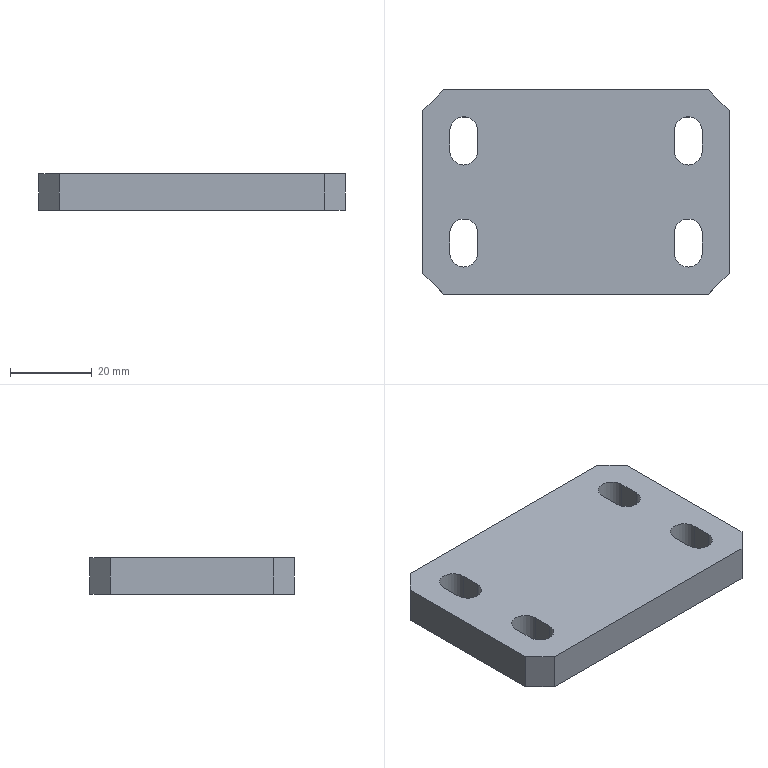Part | STEP file | [03]-6 | 1 solid | 30 faces | box 75 x 50 x 9 mm | volume 30769 mm3 | plane 18 | cylinder 12 | commonest cylinder face diameters 6.8 x12
STEP:
#1=CARTESIAN_POINT('',(65.,6.6,9.));
#2=VERTEX_POINT('',#1);
#3=CARTESIAN_POINT('',(61.6,10.,9.));
#4=VERTEX_POINT('',#3);
#5=CARTESIAN_POINT('',(65.,10.,9.));
#6=DIRECTION('',(0.,0.,-1.));
#7=DIRECTION('',(0.,-1.,0.));
#8=AXIS2_PLACEMENT_3D('',#5,#6,#7);
#9=CIRCLE('',#8,3.4);
#10=EDGE_CURVE('',#2,#4,#9,.T.);
#11=ORIENTED_EDGE('',*,*,#10,.F.);
#12=CARTESIAN_POINT('',(65.,6.6,0.));
#13=VERTEX_POINT('',#12);
#14=CARTESIAN_POINT('',(65.,6.6,9.));
#15=DIRECTION('',(0.,0.,-1.));
#16=VECTOR('',#15,1000.);
#17=LINE('',#14,#16);
#18=EDGE_CURVE('',#2,#13,#17,.T.);
#19=ORIENTED_EDGE('',*,*,#18,.T.);
#20=CARTESIAN_POINT('',(61.6,10.,0.));
#21=VERTEX_POINT('',#20);
#22=CARTESIAN_POINT('',(65.,10.,0.));
#23=DIRECTION('',(0.,0.,1.));
#24=DIRECTION('',(0.,1.,0.));
#25=AXIS2_PLACEMENT_3D('',#22,#23,#24);
#26=CIRCLE('',#25,3.4);
#27=EDGE_CURVE('',#21,#13,#26,.T.);
#28=ORIENTED_EDGE('',*,*,#27,.F.);
#29=CARTESIAN_POINT('',(61.6,10.,9.));
#30=DIRECTION('',(0.,0.,-1.));
#31=VECTOR('',#30,1000.);
#32=LINE('',#29,#31);
#33=EDGE_CURVE('',#4,#21,#32,.T.);
#34=ORIENTED_EDGE('',*,*,#33,.F.);
#35=EDGE_LOOP('',(#11,#19,#28,#34));
#36=FACE_OUTER_BOUND('',#35,.T.);
#37=CARTESIAN_POINT('',(65.,10.,9.));
#38=DIRECTION('',(0.,0.,-1.));
#39=DIRECTION('',(0.,-1.,0.));
#40=AXIS2_PLACEMENT_3D('',#37,#38,#39);
#41=CYLINDRICAL_SURFACE('',#40,3.4);
#42=ADVANCED_FACE('',(#36),#41,.F.);
#43=CARTESIAN_POINT('',(10.,31.6,9.));
#44=VERTEX_POINT('',#43);
#45=CARTESIAN_POINT('',(6.6,35.,9.));
#46=VERTEX_POINT('',#45);
#47=CARTESIAN_POINT('',(10.,35.,9.));
#48=DIRECTION('',(0.,0.,-1.));
#49=DIRECTION('',(0.,-1.,0.));
#50=AXIS2_PLACEMENT_3D('',#47,#48,#49);
#51=CIRCLE('',#50,3.4);
#52=EDGE_CURVE('',#44,#46,#51,.T.);
#53=ORIENTED_EDGE('',*,*,#52,.F.);
#54=CARTESIAN_POINT('',(10.,31.6,0.));
#55=VERTEX_POINT('',#54);
#56=CARTESIAN_POINT('',(10.,31.6,9.));
#57=DIRECTION('',(0.,0.,-1.));
#58=VECTOR('',#57,1000.);
#59=LINE('',#56,#58);
#60=EDGE_CURVE('',#44,#55,#59,.T.);
#61=ORIENTED_EDGE('',*,*,#60,.T.);
#62=CARTESIAN_POINT('',(6.6,35.,0.));
#63=VERTEX_POINT('',#62);
#64=CARTESIAN_POINT('',(10.,35.,0.));
#65=DIRECTION('',(0.,0.,1.));
#66=DIRECTION('',(0.,1.,0.));
#67=AXIS2_PLACEMENT_3D('',#64,#65,#66);
#68=CIRCLE('',#67,3.4);
#69=EDGE_CURVE('',#63,#55,#68,.T.);
#70=ORIENTED_EDGE('',*,*,#69,.F.);
#71=CARTESIAN_POINT('',(6.6,35.,9.));
#72=DIRECTION('',(0.,0.,-1.));
#73=VECTOR('',#72,1000.);
#74=LINE('',#71,#73);
#75=EDGE_CURVE('',#46,#63,#74,.T.);
#76=ORIENTED_EDGE('',*,*,#75,.F.);
#77=EDGE_LOOP('',(#53,#61,#70,#76));
#78=FACE_OUTER_BOUND('',#77,.T.);
#79=CARTESIAN_POINT('',(10.,35.,9.));
#80=DIRECTION('',(0.,0.,-1.));
#81=DIRECTION('',(0.,-1.,0.));
#82=AXIS2_PLACEMENT_3D('',#79,#80,#81);
#83=CYLINDRICAL_SURFACE('',#82,3.4);
#84=ADVANCED_FACE('',(#78),#83,.F.);
#85=CARTESIAN_POINT('',(10.,6.6,9.));
#86=VERTEX_POINT('',#85);
#87=CARTESIAN_POINT('',(6.6,10.,9.));
#88=VERTEX_POINT('',#87);
#89=CARTESIAN_POINT('',(10.,10.,9.));
#90=DIRECTION('',(0.,0.,-1.));
#91=DIRECTION('',(0.,-1.,0.));
#92=AXIS2_PLACEMENT_3D('',#89,#90,#91);
#93=CIRCLE('',#92,3.4);
#94=EDGE_CURVE('',#86,#88,#93,.T.);
#95=ORIENTED_EDGE('',*,*,#94,.F.);
#96=CARTESIAN_POINT('',(10.,6.6,0.));
#97=VERTEX_POINT('',#96);
#98=CARTESIAN_POINT('',(10.,6.6,9.));
#99=DIRECTION('',(0.,0.,-1.));
#100=VECTOR('',#99,1000.);
#101=LINE('',#98,#100);
#102=EDGE_CURVE('',#86,#97,#101,.T.);
#103=ORIENTED_EDGE('',*,*,#102,.T.);
#104=CARTESIAN_POINT('',(6.6,10.,0.));
#105=VERTEX_POINT('',#104);
#106=CARTESIAN_POINT('',(10.,10.,0.));
#107=DIRECTION('',(0.,0.,1.));
#108=DIRECTION('',(0.,1.,0.));
#109=AXIS2_PLACEMENT_3D('',#106,#107,#108);
#110=CIRCLE('',#109,3.4);
#111=EDGE_CURVE('',#105,#97,#110,.T.);
#112=ORIENTED_EDGE('',*,*,#111,.F.);
#113=CARTESIAN_POINT('',(6.6,10.,9.));
#114=DIRECTION('',(0.,0.,-1.));
#115=VECTOR('',#114,1000.);
#116=LINE('',#113,#115);
#117=EDGE_CURVE('',#88,#105,#116,.T.);
#118=ORIENTED_EDGE('',*,*,#117,.F.);
#119=EDGE_LOOP('',(#95,#103,#112,#118));
#120=FACE_OUTER_BOUND('',#119,.T.);
#121=CARTESIAN_POINT('',(10.,10.,9.));
#122=DIRECTION('',(0.,0.,-1.));
#123=DIRECTION('',(0.,-1.,0.));
#124=AXIS2_PLACEMENT_3D('',#121,#122,#123);
#125=CYLINDRICAL_SURFACE('',#124,3.4);
#126=ADVANCED_FACE('',(#120),#125,.F.);
#127=CARTESIAN_POINT('',(65.,31.6,9.));
#128=VERTEX_POINT('',#127);
#129=CARTESIAN_POINT('',(61.6,35.,9.));
#130=VERTEX_POINT('',#129);
#131=CARTESIAN_POINT('',(65.,35.,9.));
#132=DIRECTION('',(0.,0.,-1.));
#133=DIRECTION('',(0.,-1.,0.));
#134=AXIS2_PLACEMENT_3D('',#131,#132,#133);
#135=CIRCLE('',#134,3.4);
#136=EDGE_CURVE('',#128,#130,#135,.T.);
#137=ORIENTED_EDGE('',*,*,#136,.F.);
#138=CARTESIAN_POINT('',(65.,31.6,0.));
#139=VERTEX_POINT('',#138);
#140=CARTESIAN_POINT('',(65.,31.6,9.));
#141=DIRECTION('',(0.,0.,-1.));
#142=VECTOR('',#141,1000.);
#143=LINE('',#140,#142);
#144=EDGE_CURVE('',#128,#139,#143,.T.);
#145=ORIENTED_EDGE('',*,*,#144,.T.);
#146=CARTESIAN_POINT('',(61.6,35.,0.));
#147=VERTEX_POINT('',#146);
#148=CARTESIAN_POINT('',(65.,35.,0.));
#149=DIRECTION('',(0.,0.,1.));
#150=DIRECTION('',(0.,1.,0.));
#151=AXIS2_PLACEMENT_3D('',#148,#149,#150);
#152=CIRCLE('',#151,3.4);
#153=EDGE_CURVE('',#147,#139,#152,.T.);
#154=ORIENTED_EDGE('',*,*,#153,.F.);
#155=CARTESIAN_POINT('',(61.6,35.,9.));
#156=DIRECTION('',(0.,0.,-1.));
#157=VECTOR('',#156,1000.);
#158=LINE('',#155,#157);
#159=EDGE_CURVE('',#130,#147,#158,.T.);
#160=ORIENTED_EDGE('',*,*,#159,.F.);
#161=EDGE_LOOP('',(#137,#145,#154,#160));
#162=FACE_OUTER_BOUND('',#161,.T.);
#163=CARTESIAN_POINT('',(65.,35.,9.));
#164=DIRECTION('',(0.,0.,-1.));
#165=DIRECTION('',(0.,-1.,0.));
#166=AXIS2_PLACEMENT_3D('',#163,#164,#165);
#167=CYLINDRICAL_SURFACE('',#166,3.4);
#168=ADVANCED_FACE('',(#162),#167,.F.);
#169=CARTESIAN_POINT('',(0.,5.,9.));
#170=VERTEX_POINT('',#169);
#171=CARTESIAN_POINT('',(0.,45.,9.));
#172=VERTEX_POINT('',#171);
#173=CARTESIAN_POINT('',(0.,25.,9.));
#174=DIRECTION('',(0.,1.,0.));
#175=VECTOR('',#174,1000.);
#176=LINE('',#173,#175);
#177=EDGE_CURVE('',#170,#172,#176,.T.);
#178=ORIENTED_EDGE('',*,*,#177,.F.);
#179=CARTESIAN_POINT('',(5.,0.,9.));
#180=VERTEX_POINT('',#179);
#181=CARTESIAN_POINT('',(8.75,-3.75,9.));
#182=DIRECTION('',(0.7071,-0.7071,0.));
#183=VECTOR('',#182,1000.);
#184=LINE('',#181,#183);
#185=EDGE_CURVE('',#170,#180,#184,.T.);
#186=ORIENTED_EDGE('',*,*,#185,.T.);
#187=CARTESIAN_POINT('',(70.,0.,9.));
#188=VERTEX_POINT('',#187);
#189=CARTESIAN_POINT('',(37.5,0.,9.));
#190=DIRECTION('',(-1.,0.,0.));
#191=VECTOR('',#190,1000.);
#192=LINE('',#189,#191);
#193=EDGE_CURVE('',#188,#180,#192,.T.);
#194=ORIENTED_EDGE('',*,*,#193,.F.);
#195=CARTESIAN_POINT('',(75.,5.,9.));
#196=VERTEX_POINT('',#195);
#197=CARTESIAN_POINT('',(66.25,-3.75,9.));
#198=DIRECTION('',(0.7071,0.7071,0.));
#199=VECTOR('',#198,1000.);
#200=LINE('',#197,#199);
#201=EDGE_CURVE('',#188,#196,#200,.T.);
#202=ORIENTED_EDGE('',*,*,#201,.T.);
#203=CARTESIAN_POINT('',(75.,45.,9.));
#204=VERTEX_POINT('',#203);
#205=CARTESIAN_POINT('',(75.,25.,9.));
#206=DIRECTION('',(0.,-1.,0.));
#207=VECTOR('',#206,1000.);
#208=LINE('',#205,#207);
#209=EDGE_CURVE('',#204,#196,#208,.T.);
#210=ORIENTED_EDGE('',*,*,#209,.F.);
#211=CARTESIAN_POINT('',(70.,50.,9.));
#212=VERTEX_POINT('',#211);
#213=CARTESIAN_POINT('',(66.25,53.75,9.));
#214=DIRECTION('',(-0.7071,0.7071,0.));
#215=VECTOR('',#214,1000.);
#216=LINE('',#213,#215);
#217=EDGE_CURVE('',#204,#212,#216,.T.);
#218=ORIENTED_EDGE('',*,*,#217,.T.);
#219=CARTESIAN_POINT('',(5.,50.,9.));
#220=VERTEX_POINT('',#219);
#221=CARTESIAN_POINT('',(37.5,50.,9.));
#222=DIRECTION('',(1.,0.,0.));
#223=VECTOR('',#222,1000.);
#224=LINE('',#221,#223);
#225=EDGE_CURVE('',#220,#212,#224,.T.);
#226=ORIENTED_EDGE('',*,*,#225,.F.);
#227=CARTESIAN_POINT('',(8.75,53.75,9.));
#228=DIRECTION('',(-0.7071,-0.7071,0.));
#229=VECTOR('',#228,1000.);
#230=LINE('',#227,#229);
#231=EDGE_CURVE('',#220,#172,#230,.T.);
#232=ORIENTED_EDGE('',*,*,#231,.T.);
#233=EDGE_LOOP('',(#178,#186,#194,#202,#210,#218,#226,#232));
#234=FACE_OUTER_BOUND('',#233,.T.);
#235=CARTESIAN_POINT('',(68.4,40.,9.));
#236=VERTEX_POINT('',#235);
#237=CARTESIAN_POINT('',(68.4,35.,9.));
#238=VERTEX_POINT('',#237);
#239=CARTESIAN_POINT('',(68.4,37.5,9.));
#240=DIRECTION('',(0.,-1.,0.));
#241=VECTOR('',#240,1000.);
#242=LINE('',#239,#241);
#243=EDGE_CURVE('',#236,#238,#242,.T.);
#244=ORIENTED_EDGE('',*,*,#243,.T.);
#245=CARTESIAN_POINT('',(65.,35.,9.));
#246=DIRECTION('',(0.,0.,-1.));
#247=DIRECTION('',(0.,-1.,0.));
#248=AXIS2_PLACEMENT_3D('',#245,#246,#247);
#249=CIRCLE('',#248,3.4);
#250=EDGE_CURVE('',#238,#128,#249,.T.);
#251=ORIENTED_EDGE('',*,*,#250,.T.);
#252=ORIENTED_EDGE('',*,*,#136,.T.);
#253=CARTESIAN_POINT('',(61.6,40.,9.));
#254=VERTEX_POINT('',#253);
#255=CARTESIAN_POINT('',(61.6,37.5,9.));
#256=DIRECTION('',(0.,1.,0.));
#257=VECTOR('',#256,1000.);
#258=LINE('',#255,#257);
#259=EDGE_CURVE('',#130,#254,#258,.T.);
#260=ORIENTED_EDGE('',*,*,#259,.T.);
#261=CARTESIAN_POINT('',(65.,40.,9.));
#262=DIRECTION('',(0.,0.,-1.));
#263=DIRECTION('',(0.,-1.,0.));
#264=AXIS2_PLACEMENT_3D('',#261,#262,#263);
#265=CIRCLE('',#264,3.4);
#266=EDGE_CURVE('',#254,#236,#265,.T.);
#267=ORIENTED_EDGE('',*,*,#266,.T.);
#268=EDGE_LOOP('',(#244,#251,#252,#260,#267));
#269=FACE_BOUND('',#268,.T.);
#270=CARTESIAN_POINT('',(13.4,15.,9.));
#271=VERTEX_POINT('',#270);
#272=CARTESIAN_POINT('',(13.4,10.,9.));
#273=VERTEX_POINT('',#272);
#274=CARTESIAN_POINT('',(13.4,12.5,9.));
#275=DIRECTION('',(0.,-1.,0.));
#276=VECTOR('',#275,1000.);
#277=LINE('',#274,#276);
#278=EDGE_CURVE('',#271,#273,#277,.T.);
#279=ORIENTED_EDGE('',*,*,#278,.T.);
#280=CARTESIAN_POINT('',(10.,10.,9.));
#281=DIRECTION('',(0.,0.,-1.));
#282=DIRECTION('',(0.,-1.,0.));
#283=AXIS2_PLACEMENT_3D('',#280,#281,#282);
#284=CIRCLE('',#283,3.4);
#285=EDGE_CURVE('',#273,#86,#284,.T.);
#286=ORIENTED_EDGE('',*,*,#285,.T.);
#287=ORIENTED_EDGE('',*,*,#94,.T.);
#288=CARTESIAN_POINT('',(6.6,15.,9.));
#289=VERTEX_POINT('',#288);
#290=CARTESIAN_POINT('',(6.6,12.5,9.));
#291=DIRECTION('',(0.,1.,0.));
#292=VECTOR('',#291,1000.);
#293=LINE('',#290,#292);
#294=EDGE_CURVE('',#88,#289,#293,.T.);
#295=ORIENTED_EDGE('',*,*,#294,.T.);
#296=CARTESIAN_POINT('',(10.,15.,9.));
#297=DIRECTION('',(0.,0.,-1.));
#298=DIRECTION('',(0.,-1.,0.));
#299=AXIS2_PLACEMENT_3D('',#296,#297,#298);
#300=CIRCLE('',#299,3.4);
#301=EDGE_CURVE('',#289,#271,#300,.T.);
#302=ORIENTED_EDGE('',*,*,#301,.T.);
#303=EDGE_LOOP('',(#279,#286,#287,#295,#302));
#304=FACE_BOUND('',#303,.T.);
#305=CARTESIAN_POINT('',(13.4,40.,9.));
#306=VERTEX_POINT('',#305);
#307=CARTESIAN_POINT('',(13.4,35.,9.));
#308=VERTEX_POINT('',#307);
#309=CARTESIAN_POINT('',(13.4,37.5,9.));
#310=DIRECTION('',(0.,-1.,0.));
#311=VECTOR('',#310,1000.);
#312=LINE('',#309,#311);
#313=EDGE_CURVE('',#306,#308,#312,.T.);
#314=ORIENTED_EDGE('',*,*,#313,.T.);
#315=CARTESIAN_POINT('',(10.,35.,9.));
#316=DIRECTION('',(0.,0.,-1.));
#317=DIRECTION('',(0.,-1.,0.));
#318=AXIS2_PLACEMENT_3D('',#315,#316,#317);
#319=CIRCLE('',#318,3.4);
#320=EDGE_CURVE('',#308,#44,#319,.T.);
#321=ORIENTED_EDGE('',*,*,#320,.T.);
#322=ORIENTED_EDGE('',*,*,#52,.T.);
#323=CARTESIAN_POINT('',(6.6,40.,9.));
#324=VERTEX_POINT('',#323);
#325=CARTESIAN_POINT('',(6.6,37.5,9.));
#326=DIRECTION('',(0.,1.,0.));
#327=VECTOR('',#326,1000.);
#328=LINE('',#325,#327);
#329=EDGE_CURVE('',#46,#324,#328,.T.);
#330=ORIENTED_EDGE('',*,*,#329,.T.);
#331=CARTESIAN_POINT('',(10.,40.,9.));
#332=DIRECTION('',(0.,0.,-1.));
#333=DIRECTION('',(0.,-1.,0.));
#334=AXIS2_PLACEMENT_3D('',#331,#332,#333);
#335=CIRCLE('',#334,3.4);
#336=EDGE_CURVE('',#324,#306,#335,.T.);
#337=ORIENTED_EDGE('',*,*,#336,.T.);
#338=EDGE_LOOP('',(#314,#321,#322,#330,#337));
#339=FACE_BOUND('',#338,.T.);
#340=CARTESIAN_POINT('',(68.4,15.,9.));
#341=VERTEX_POINT('',#340);
#342=CARTESIAN_POINT('',(68.4,10.,9.));
#343=VERTEX_POINT('',#342);
#344=CARTESIAN_POINT('',(68.4,12.5,9.));
#345=DIRECTION('',(0.,-1.,0.));
#346=VECTOR('',#345,1000.);
#347=LINE('',#344,#346);
#348=EDGE_CURVE('',#341,#343,#347,.T.);
#349=ORIENTED_EDGE('',*,*,#348,.T.);
#350=CARTESIAN_POINT('',(65.,10.,9.));
#351=DIRECTION('',(0.,0.,-1.));
#352=DIRECTION('',(0.,-1.,0.));
#353=AXIS2_PLACEMENT_3D('',#350,#351,#352);
#354=CIRCLE('',#353,3.4);
#355=EDGE_CURVE('',#343,#2,#354,.T.);
#356=ORIENTED_EDGE('',*,*,#355,.T.);
#357=ORIENTED_EDGE('',*,*,#10,.T.);
#358=CARTESIAN_POINT('',(61.6,15.,9.));
#359=VERTEX_POINT('',#358);
#360=CARTESIAN_POINT('',(61.6,12.5,9.));
#361=DIRECTION('',(0.,1.,0.));
#362=VECTOR('',#361,1000.);
#363=LINE('',#360,#362);
#364=EDGE_CURVE('',#4,#359,#363,.T.);
#365=ORIENTED_EDGE('',*,*,#364,.T.);
#366=CARTESIAN_POINT('',(65.,15.,9.));
#367=DIRECTION('',(0.,0.,-1.));
#368=DIRECTION('',(0.,-1.,0.));
#369=AXIS2_PLACEMENT_3D('',#366,#367,#368);
#370=CIRCLE('',#369,3.4);
#371=EDGE_CURVE('',#359,#341,#370,.T.);
#372=ORIENTED_EDGE('',*,*,#371,.T.);
#373=EDGE_LOOP('',(#349,#356,#357,#365,#372));
#374=FACE_BOUND('',#373,.T.);
#375=CARTESIAN_POINT('',(37.5,25.,9.));
#376=DIRECTION('',(0.,0.,1.));
#377=DIRECTION('',(1.,0.,0.));
#378=AXIS2_PLACEMENT_3D('',#375,#376,#377);
#379=PLANE('',#378);
#380=ADVANCED_FACE('',(#234,#269,#304,#339,#374),#379,.T.);
#381=CARTESIAN_POINT('',(5.,0.,0.));
#382=VERTEX_POINT('',#381);
#383=CARTESIAN_POINT('',(70.,0.,0.));
#384=VERTEX_POINT('',#383);
#385=CARTESIAN_POINT('',(37.5,0.,0.));
#386=DIRECTION('',(1.,0.,0.));
#387=VECTOR('',#386,1000.);
#388=LINE('',#385,#387);
#389=EDGE_CURVE('',#382,#384,#388,.T.);
#390=ORIENTED_EDGE('',*,*,#389,.F.);
#391=CARTESIAN_POINT('',(0.,5.,0.));
#392=VERTEX_POINT('',#391);
#393=CARTESIAN_POINT('',(8.75,-3.75,0.));
#394=DIRECTION('',(-0.7071,0.7071,0.));
#395=VECTOR('',#394,1000.);
#396=LINE('',#393,#395);
#397=EDGE_CURVE('',#382,#392,#396,.T.);
#398=ORIENTED_EDGE('',*,*,#397,.T.);
#399=CARTESIAN_POINT('',(0.,45.,0.));
#400=VERTEX_POINT('',#399);
#401=CARTESIAN_POINT('',(0.,25.,0.));
#402=DIRECTION('',(0.,-1.,0.));
#403=VECTOR('',#402,1000.);
#404=LINE('',#401,#403);
#405=EDGE_CURVE('',#400,#392,#404,.T.);
#406=ORIENTED_EDGE('',*,*,#405,.F.);
#407=CARTESIAN_POINT('',(5.,50.,0.));
#408=VERTEX_POINT('',#407);
#409=CARTESIAN_POINT('',(8.75,53.75,0.));
#410=DIRECTION('',(0.7071,0.7071,0.));
#411=VECTOR('',#410,1000.);
#412=LINE('',#409,#411);
#413=EDGE_CURVE('',#400,#408,#412,.T.);
#414=ORIENTED_EDGE('',*,*,#413,.T.);
#415=CARTESIAN_POINT('',(70.,50.,0.));
#416=VERTEX_POINT('',#415);
#417=CARTESIAN_POINT('',(37.5,50.,0.));
#418=DIRECTION('',(-1.,0.,0.));
#419=VECTOR('',#418,1000.);
#420=LINE('',#417,#419);
#421=EDGE_CURVE('',#416,#408,#420,.T.);
#422=ORIENTED_EDGE('',*,*,#421,.F.);
#423=CARTESIAN_POINT('',(75.,45.,0.));
#424=VERTEX_POINT('',#423);
#425=CARTESIAN_POINT('',(66.25,53.75,0.));
#426=DIRECTION('',(0.7071,-0.7071,0.));
#427=VECTOR('',#426,1000.);
#428=LINE('',#425,#427);
#429=EDGE_CURVE('',#416,#424,#428,.T.);
#430=ORIENTED_EDGE('',*,*,#429,.T.);
#431=CARTESIAN_POINT('',(75.,5.,0.));
#432=VERTEX_POINT('',#431);
#433=CARTESIAN_POINT('',(75.,25.,0.));
#434=DIRECTION('',(0.,1.,0.));
#435=VECTOR('',#434,1000.);
#436=LINE('',#433,#435);
#437=EDGE_CURVE('',#432,#424,#436,.T.);
#438=ORIENTED_EDGE('',*,*,#437,.F.);
#439=CARTESIAN_POINT('',(66.25,-3.75,0.));
#440=DIRECTION('',(-0.7071,-0.7071,0.));
#441=VECTOR('',#440,1000.);
#442=LINE('',#439,#441);
#443=EDGE_CURVE('',#432,#384,#442,.T.);
#444=ORIENTED_EDGE('',*,*,#443,.T.);
#445=EDGE_LOOP('',(#390,#398,#406,#414,#422,#430,#438,#444));
#446=FACE_OUTER_BOUND('',#445,.T.);
#447=CARTESIAN_POINT('',(61.6,40.,0.));
#448=VERTEX_POINT('',#447);
#449=CARTESIAN_POINT('',(61.6,37.5,0.));
#450=DIRECTION('',(0.,-1.,0.));
#451=VECTOR('',#450,1000.);
#452=LINE('',#449,#451);
#453=EDGE_CURVE('',#448,#147,#452,.T.);
#454=ORIENTED_EDGE('',*,*,#453,.T.);
#455=ORIENTED_EDGE('',*,*,#153,.T.);
#456=CARTESIAN_POINT('',(68.4,35.,0.));
#457=VERTEX_POINT('',#456);
#458=CARTESIAN_POINT('',(65.,35.,0.));
#459=DIRECTION('',(0.,0.,1.));
#460=DIRECTION('',(0.,1.,0.));
#461=AXIS2_PLACEMENT_3D('',#458,#459,#460);
#462=CIRCLE('',#461,3.4);
#463=EDGE_CURVE('',#139,#457,#462,.T.);
#464=ORIENTED_EDGE('',*,*,#463,.T.);
#465=CARTESIAN_POINT('',(68.4,40.,0.));
#466=VERTEX_POINT('',#465);
#467=CARTESIAN_POINT('',(68.4,37.5,0.));
#468=DIRECTION('',(0.,1.,0.));
#469=VECTOR('',#468,1000.);
#470=LINE('',#467,#469);
#471=EDGE_CURVE('',#457,#466,#470,.T.);
#472=ORIENTED_EDGE('',*,*,#471,.T.);
#473=CARTESIAN_POINT('',(65.,40.,0.));
#474=DIRECTION('',(0.,0.,1.));
#475=DIRECTION('',(0.,1.,0.));
#476=AXIS2_PLACEMENT_3D('',#473,#474,#475);
#477=CIRCLE('',#476,3.4);
#478=EDGE_CURVE('',#466,#448,#477,.T.);
#479=ORIENTED_EDGE('',*,*,#478,.T.);
#480=EDGE_LOOP('',(#454,#455,#464,#472,#479));
#481=FACE_BOUND('',#480,.T.);
#482=CARTESIAN_POINT('',(6.6,15.,0.));
#483=VERTEX_POINT('',#482);
#484=CARTESIAN_POINT('',(6.6,12.5,0.));
#485=DIRECTION('',(0.,-1.,0.));
#486=VECTOR('',#485,1000.);
#487=LINE('',#484,#486);
#488=EDGE_CURVE('',#483,#105,#487,.T.);
#489=ORIENTED_EDGE('',*,*,#488,.T.);
#490=ORIENTED_EDGE('',*,*,#111,.T.);
#491=CARTESIAN_POINT('',(13.4,10.,0.));
#492=VERTEX_POINT('',#491);
#493=CARTESIAN_POINT('',(10.,10.,0.));
#494=DIRECTION('',(0.,0.,1.));
#495=DIRECTION('',(0.,1.,0.));
#496=AXIS2_PLACEMENT_3D('',#493,#494,#495);
#497=CIRCLE('',#496,3.4);
#498=EDGE_CURVE('',#97,#492,#497,.T.);
#499=ORIENTED_EDGE('',*,*,#498,.T.);
#500=CARTESIAN_POINT('',(13.4,15.,0.));
#501=VERTEX_POINT('',#500);
#502=CARTESIAN_POINT('',(13.4,12.5,0.));
#503=DIRECTION('',(0.,1.,0.));
#504=VECTOR('',#503,1000.);
#505=LINE('',#502,#504);
#506=EDGE_CURVE('',#492,#501,#505,.T.);
#507=ORIENTED_EDGE('',*,*,#506,.T.);
#508=CARTESIAN_POINT('',(10.,15.,0.));
#509=DIRECTION('',(0.,0.,1.));
#510=DIRECTION('',(0.,1.,0.));
#511=AXIS2_PLACEMENT_3D('',#508,#509,#510);
#512=CIRCLE('',#511,3.4);
#513=EDGE_CURVE('',#501,#483,#512,.T.);
#514=ORIENTED_EDGE('',*,*,#513,.T.);
#515=EDGE_LOOP('',(#489,#490,#499,#507,#514));
#516=FACE_BOUND('',#515,.T.);
#517=CARTESIAN_POINT('',(6.6,40.,0.));
#518=VERTEX_POINT('',#517);
#519=CARTESIAN_POINT('',(6.6,37.5,0.));
#520=DIRECTION('',(0.,-1.,0.));
#521=VECTOR('',#520,1000.);
#522=LINE('',#519,#521);
#523=EDGE_CURVE('',#518,#63,#522,.T.);
#524=ORIENTED_EDGE('',*,*,#523,.T.);
#525=ORIENTED_EDGE('',*,*,#69,.T.);
#526=CARTESIAN_POINT('',(13.4,35.,0.));
#527=VERTEX_POINT('',#526);
#528=CARTESIAN_POINT('',(10.,35.,0.));
#529=DIRECTION('',(0.,0.,1.));
#530=DIRECTION('',(0.,1.,0.));
#531=AXIS2_PLACEMENT_3D('',#528,#529,#530);
#532=CIRCLE('',#531,3.4);
#533=EDGE_CURVE('',#55,#527,#532,.T.);
#534=ORIENTED_EDGE('',*,*,#533,.T.);
#535=CARTESIAN_POINT('',(13.4,40.,0.));
#536=VERTEX_POINT('',#535);
#537=CARTESIAN_POINT('',(13.4,37.5,0.));
#538=DIRECTION('',(0.,1.,0.));
#539=VECTOR('',#538,1000.);
#540=LINE('',#537,#539);
#541=EDGE_CURVE('',#527,#536,#540,.T.);
#542=ORIENTED_EDGE('',*,*,#541,.T.);
#543=CARTESIAN_POINT('',(10.,40.,0.));
#544=DIRECTION('',(0.,0.,1.));
#545=DIRECTION('',(0.,1.,0.));
#546=AXIS2_PLACEMENT_3D('',#543,#544,#545);
#547=CIRCLE('',#546,3.4);
#548=EDGE_CURVE('',#536,#518,#547,.T.);
#549=ORIENTED_EDGE('',*,*,#548,.T.);
#550=EDGE_LOOP('',(#524,#525,#534,#542,#549));
#551=FACE_BOUND('',#550,.T.);
#552=CARTESIAN_POINT('',(61.6,15.,0.));
#553=VERTEX_POINT('',#552);
#554=CARTESIAN_POINT('',(61.6,12.5,0.));
#555=DIRECTION('',(0.,-1.,0.));
#556=VECTOR('',#555,1000.);
#557=LINE('',#554,#556);
#558=EDGE_CURVE('',#553,#21,#557,.T.);
#559=ORIENTED_EDGE('',*,*,#558,.T.);
#560=ORIENTED_EDGE('',*,*,#27,.T.);
#561=CARTESIAN_POINT('',(68.4,10.,0.));
#562=VERTEX_POINT('',#561);
#563=CARTESIAN_POINT('',(65.,10.,0.));
#564=DIRECTION('',(0.,0.,1.));
#565=DIRECTION('',(0.,1.,0.));
#566=AXIS2_PLACEMENT_3D('',#563,#564,#565);
#567=CIRCLE('',#566,3.4);
#568=EDGE_CURVE('',#13,#562,#567,.T.);
#569=ORIENTED_EDGE('',*,*,#568,.T.);
#570=CARTESIAN_POINT('',(68.4,15.,0.));
#571=VERTEX_POINT('',#570);
#572=CARTESIAN_POINT('',(68.4,12.5,0.));
#573=DIRECTION('',(0.,1.,0.));
#574=VECTOR('',#573,1000.);
#575=LINE('',#572,#574);
#576=EDGE_CURVE('',#562,#571,#575,.T.);
#577=ORIENTED_EDGE('',*,*,#576,.T.);
#578=CARTESIAN_POINT('',(65.,15.,0.));
#579=DIRECTION('',(0.,0.,1.));
#580=DIRECTION('',(0.,1.,0.));
#581=AXIS2_PLACEMENT_3D('',#578,#579,#580);
#582=CIRCLE('',#581,3.4);
#583=EDGE_CURVE('',#571,#553,#582,.T.);
#584=ORIENTED_EDGE('',*,*,#583,.T.);
#585=EDGE_LOOP('',(#559,#560,#569,#577,#584));
#586=FACE_BOUND('',#585,.T.);
#587=CARTESIAN_POINT('',(37.5,25.,0.));
#588=DIRECTION('',(0.,0.,-1.));
#589=DIRECTION('',(-1.,0.,0.));
#590=AXIS2_PLACEMENT_3D('',#587,#588,#589);
#591=PLANE('',#590);
#592=ADVANCED_FACE('',(#446,#481,#516,#551,#586),#591,.T.);
#593=ORIENTED_EDGE('',*,*,#193,.T.);
#594=CARTESIAN_POINT('',(5.,0.,0.));
#595=DIRECTION('',(0.,0.,-1.));
#596=VECTOR('',#595,1000.);
#597=LINE('',#594,#596);
#598=EDGE_CURVE('',#180,#382,#597,.T.);
#599=ORIENTED_EDGE('',*,*,#598,.T.);
#600=ORIENTED_EDGE('',*,*,#389,.T.);
#601=CARTESIAN_POINT('',(70.,0.,0.));
#602=DIRECTION('',(0.,0.,1.));
#603=VECTOR('',#602,1000.);
#604=LINE('',#601,#603);
#605=EDGE_CURVE('',#384,#188,#604,.T.);
#606=ORIENTED_EDGE('',*,*,#605,.T.);
#607=EDGE_LOOP('',(#593,#599,#600,#606));
#608=FACE_OUTER_BOUND('',#607,.T.);
#609=CARTESIAN_POINT('',(37.5,0.,0.));
#610=DIRECTION('',(0.,-1.,0.));
#611=DIRECTION('',(0.,0.,-1.));
#612=AXIS2_PLACEMENT_3D('',#609,#610,#611);
#613=PLANE('',#612);
#614=ADVANCED_FACE('',(#608),#613,.T.);
#615=ORIENTED_EDGE('',*,*,#405,.T.);
#616=CARTESIAN_POINT('',(0.,5.,0.));
#617=DIRECTION('',(0.,0.,1.));
#618=VECTOR('',#617,1000.);
#619=LINE('',#616,#618);
#620=EDGE_CURVE('',#392,#170,#619,.T.);
#621=ORIENTED_EDGE('',*,*,#620,.T.);
#622=ORIENTED_EDGE('',*,*,#177,.T.);
#623=CARTESIAN_POINT('',(0.,45.,0.));
#624=DIRECTION('',(0.,0.,-1.));
#625=VECTOR('',#624,1000.);
#626=LINE('',#623,#625);
#627=EDGE_CURVE('',#172,#400,#626,.T.);
#628=ORIENTED_EDGE('',*,*,#627,.T.);
#629=EDGE_LOOP('',(#615,#621,#622,#628));
#630=FACE_OUTER_BOUND('',#629,.T.);
#631=CARTESIAN_POINT('',(0.,25.,0.));
#632=DIRECTION('',(-1.,0.,0.));
#633=DIRECTION('',(0.,0.,1.));
#634=AXIS2_PLACEMENT_3D('',#631,#632,#633);
#635=PLANE('',#634);
#636=ADVANCED_FACE('',(#630),#635,.T.);
#637=ORIENTED_EDGE('',*,*,#421,.T.);
#638=CARTESIAN_POINT('',(5.,50.,0.));
#639=DIRECTION('',(0.,0.,1.));
#640=VECTOR('',#639,1000.);
#641=LINE('',#638,#640);
#642=EDGE_CURVE('',#408,#220,#641,.T.);
#643=ORIENTED_EDGE('',*,*,#642,.T.);
#644=ORIENTED_EDGE('',*,*,#225,.T.);
#645=CARTESIAN_POINT('',(70.,50.,0.));
#646=DIRECTION('',(0.,0.,-1.));
#647=VECTOR('',#646,1000.);
#648=LINE('',#645,#647);
#649=EDGE_CURVE('',#212,#416,#648,.T.);
#650=ORIENTED_EDGE('',*,*,#649,.T.);
#651=EDGE_LOOP('',(#637,#643,#644,#650));
#652=FACE_OUTER_BOUND('',#651,.T.);
#653=CARTESIAN_POINT('',(37.5,50.,0.));
#654=DIRECTION('',(0.,1.,0.));
#655=DIRECTION('',(0.,0.,1.));
#656=AXIS2_PLACEMENT_3D('',#653,#654,#655);
#657=PLANE('',#656);
#658=ADVANCED_FACE('',(#652),#657,.T.);
#659=ORIENTED_EDGE('',*,*,#209,.T.);
#660=CARTESIAN_POINT('',(75.,5.,0.));
#661=DIRECTION('',(0.,0.,-1.));
#662=VECTOR('',#661,1000.);
#663=LINE('',#660,#662);
#664=EDGE_CURVE('',#196,#432,#663,.T.);
#665=ORIENTED_EDGE('',*,*,#664,.T.);
#666=ORIENTED_EDGE('',*,*,#437,.T.);
#667=CARTESIAN_POINT('',(75.,45.,0.));
#668=DIRECTION('',(0.,0.,1.));
#669=VECTOR('',#668,1000.);
#670=LINE('',#667,#669);
#671=EDGE_CURVE('',#424,#204,#670,.T.);
#672=ORIENTED_EDGE('',*,*,#671,.T.);
#673=EDGE_LOOP('',(#659,#665,#666,#672));
#674=FACE_OUTER_BOUND('',#673,.T.);
#675=CARTESIAN_POINT('',(75.,25.,0.));
#676=DIRECTION('',(1.,0.,0.));
#677=DIRECTION('',(0.,0.,-1.));
#678=AXIS2_PLACEMENT_3D('',#675,#676,#677);
#679=PLANE('',#678);
#680=ADVANCED_FACE('',(#674),#679,.T.);
#681=ORIENTED_EDGE('',*,*,#429,.F.);
#682=ORIENTED_EDGE('',*,*,#649,.F.);
#683=ORIENTED_EDGE('',*,*,#217,.F.);
#684=ORIENTED_EDGE('',*,*,#671,.F.);
#685=EDGE_LOOP('',(#681,#682,#683,#684));
#686=FACE_OUTER_BOUND('',#685,.T.);
#687=CARTESIAN_POINT('',(75.,45.,0.));
#688=DIRECTION('',(-0.7071,-0.7071,0.));
#689=DIRECTION('',(0.,0.,1.));
#690=AXIS2_PLACEMENT_3D('',#687,#688,#689);
#691=PLANE('',#690);
#692=ADVANCED_FACE('',(#686),#691,.F.);
#693=ORIENTED_EDGE('',*,*,#443,.F.);
#694=ORIENTED_EDGE('',*,*,#664,.F.);
#695=ORIENTED_EDGE('',*,*,#201,.F.);
#696=ORIENTED_EDGE('',*,*,#605,.F.);
#697=EDGE_LOOP('',(#693,#694,#695,#696));
#698=FACE_OUTER_BOUND('',#697,.T.);
#699=CARTESIAN_POINT('',(70.,0.,0.));
#700=DIRECTION('',(-0.7071,0.7071,0.));
#701=DIRECTION('',(0.,0.,1.));
#702=AXIS2_PLACEMENT_3D('',#699,#700,#701);
#703=PLANE('',#702);
#704=ADVANCED_FACE('',(#698),#703,.F.);
#705=ORIENTED_EDGE('',*,*,#413,.F.);
#706=ORIENTED_EDGE('',*,*,#627,.F.);
#707=ORIENTED_EDGE('',*,*,#231,.F.);
#708=ORIENTED_EDGE('',*,*,#642,.F.);
#709=EDGE_LOOP('',(#705,#706,#707,#708));
#710=FACE_OUTER_BOUND('',#709,.T.);
#711=CARTESIAN_POINT('',(5.,50.,0.));
#712=DIRECTION('',(0.7071,-0.7071,0.));
#713=DIRECTION('',(0.,0.,1.));
#714=AXIS2_PLACEMENT_3D('',#711,#712,#713);
#715=PLANE('',#714);
#716=ADVANCED_FACE('',(#710),#715,.F.);
#717=ORIENTED_EDGE('',*,*,#397,.F.);
#718=ORIENTED_EDGE('',*,*,#598,.F.);
#719=ORIENTED_EDGE('',*,*,#185,.F.);
#720=ORIENTED_EDGE('',*,*,#620,.F.);
#721=EDGE_LOOP('',(#717,#718,#719,#720));
#722=FACE_OUTER_BOUND('',#721,.T.);
#723=CARTESIAN_POINT('',(0.,5.,0.));
#724=DIRECTION('',(0.7071,0.7071,0.));
#725=DIRECTION('',(0.,0.,1.));
#726=AXIS2_PLACEMENT_3D('',#723,#724,#725);
#727=PLANE('',#726);
#728=ADVANCED_FACE('',(#722),#727,.F.);
#729=CARTESIAN_POINT('',(68.4,35.,9.));
#730=DIRECTION('',(0.,0.,-1.));
#731=VECTOR('',#730,1000.);
#732=LINE('',#729,#731);
#733=EDGE_CURVE('',#238,#457,#732,.T.);
#734=ORIENTED_EDGE('',*,*,#733,.F.);
#735=ORIENTED_EDGE('',*,*,#243,.F.);
#736=CARTESIAN_POINT('',(68.4,40.,9.));
#737=DIRECTION('',(0.,0.,-1.));
#738=VECTOR('',#737,1000.);
#739=LINE('',#736,#738);
#740=EDGE_CURVE('',#236,#466,#739,.T.);
#741=ORIENTED_EDGE('',*,*,#740,.T.);
#742=ORIENTED_EDGE('',*,*,#471,.F.);
#743=EDGE_LOOP('',(#734,#735,#741,#742));
#744=FACE_OUTER_BOUND('',#743,.T.);
#745=CARTESIAN_POINT('',(68.4,37.5,9.));
#746=DIRECTION('',(1.,0.,0.));
#747=DIRECTION('',(0.,0.,1.));
#748=AXIS2_PLACEMENT_3D('',#745,#746,#747);
#749=PLANE('',#748);
#750=ADVANCED_FACE('',(#744),#749,.F.);
#751=CARTESIAN_POINT('',(61.6,40.,9.));
#752=DIRECTION('',(0.,0.,-1.));
#753=VECTOR('',#752,1000.);
#754=LINE('',#751,#753);
#755=EDGE_CURVE('',#254,#448,#754,.T.);
#756=ORIENTED_EDGE('',*,*,#755,.F.);
#757=ORIENTED_EDGE('',*,*,#259,.F.);
#758=ORIENTED_EDGE('',*,*,#159,.T.);
#759=ORIENTED_EDGE('',*,*,#453,.F.);
#760=EDGE_LOOP('',(#756,#757,#758,#759));
#761=FACE_OUTER_BOUND('',#760,.T.);
#762=CARTESIAN_POINT('',(61.6,37.5,9.));
#763=DIRECTION('',(-1.,0.,0.));
#764=DIRECTION('',(0.,0.,-1.));
#765=AXIS2_PLACEMENT_3D('',#762,#763,#764);
#766=PLANE('',#765);
#767=ADVANCED_FACE('',(#761),#766,.F.);
#768=ORIENTED_EDGE('',*,*,#144,.F.);
#769=ORIENTED_EDGE('',*,*,#250,.F.);
#770=ORIENTED_EDGE('',*,*,#733,.T.);
#771=ORIENTED_EDGE('',*,*,#463,.F.);
#772=EDGE_LOOP('',(#768,#769,#770,#771));
#773=FACE_OUTER_BOUND('',#772,.T.);
#774=CARTESIAN_POINT('',(65.,35.,9.));
#775=DIRECTION('',(0.,0.,-1.));
#776=DIRECTION('',(0.,-1.,0.));
#777=AXIS2_PLACEMENT_3D('',#774,#775,#776);
#778=CYLINDRICAL_SURFACE('',#777,3.4);
#779=ADVANCED_FACE('',(#773),#778,.F.);
#780=ORIENTED_EDGE('',*,*,#266,.F.);
#781=ORIENTED_EDGE('',*,*,#755,.T.);
#782=ORIENTED_EDGE('',*,*,#478,.F.);
#783=ORIENTED_EDGE('',*,*,#740,.F.);
#784=EDGE_LOOP('',(#780,#781,#782,#783));
#785=FACE_OUTER_BOUND('',#784,.T.);
#786=CARTESIAN_POINT('',(65.,40.,9.));
#787=DIRECTION('',(0.,0.,-1.));
#788=DIRECTION('',(0.,-1.,0.));
#789=AXIS2_PLACEMENT_3D('',#786,#787,#788);
#790=CYLINDRICAL_SURFACE('',#789,3.4);
#791=ADVANCED_FACE('',(#785),#790,.F.);
#792=CARTESIAN_POINT('',(13.4,10.,9.));
#793=DIRECTION('',(0.,0.,-1.));
#794=VECTOR('',#793,1000.);
#795=LINE('',#792,#794);
#796=EDGE_CURVE('',#273,#492,#795,.T.);
#797=ORIENTED_EDGE('',*,*,#796,.F.);
#798=ORIENTED_EDGE('',*,*,#278,.F.);
#799=CARTESIAN_POINT('',(13.4,15.,9.));
#800=DIRECTION('',(0.,0.,-1.));
#801=VECTOR('',#800,1000.);
#802=LINE('',#799,#801);
#803=EDGE_CURVE('',#271,#501,#802,.T.);
#804=ORIENTED_EDGE('',*,*,#803,.T.);
#805=ORIENTED_EDGE('',*,*,#506,.F.);
#806=EDGE_LOOP('',(#797,#798,#804,#805));
#807=FACE_OUTER_BOUND('',#806,.T.);
#808=CARTESIAN_POINT('',(13.4,12.5,9.));
#809=DIRECTION('',(1.,0.,0.));
#810=DIRECTION('',(0.,0.,1.));
#811=AXIS2_PLACEMENT_3D('',#808,#809,#810);
#812=PLANE('',#811);
#813=ADVANCED_FACE('',(#807),#812,.F.);
#814=CARTESIAN_POINT('',(6.6,15.,9.));
#815=DIRECTION('',(0.,0.,-1.));
#816=VECTOR('',#815,1000.);
#817=LINE('',#814,#816);
#818=EDGE_CURVE('',#289,#483,#817,.T.);
#819=ORIENTED_EDGE('',*,*,#818,.F.);
#820=ORIENTED_EDGE('',*,*,#294,.F.);
#821=ORIENTED_EDGE('',*,*,#117,.T.);
#822=ORIENTED_EDGE('',*,*,#488,.F.);
#823=EDGE_LOOP('',(#819,#820,#821,#822));
#824=FACE_OUTER_BOUND('',#823,.T.);
#825=CARTESIAN_POINT('',(6.6,12.5,9.));
#826=DIRECTION('',(-1.,0.,0.));
#827=DIRECTION('',(0.,0.,-1.));
#828=AXIS2_PLACEMENT_3D('',#825,#826,#827);
#829=PLANE('',#828);
#830=ADVANCED_FACE('',(#824),#829,.F.);
#831=ORIENTED_EDGE('',*,*,#102,.F.);
#832=ORIENTED_EDGE('',*,*,#285,.F.);
#833=ORIENTED_EDGE('',*,*,#796,.T.);
#834=ORIENTED_EDGE('',*,*,#498,.F.);
#835=EDGE_LOOP('',(#831,#832,#833,#834));
#836=FACE_OUTER_BOUND('',#835,.T.);
#837=CARTESIAN_POINT('',(10.,10.,9.));
#838=DIRECTION('',(0.,0.,-1.));
#839=DIRECTION('',(0.,-1.,0.));
#840=AXIS2_PLACEMENT_3D('',#837,#838,#839);
#841=CYLINDRICAL_SURFACE('',#840,3.4);
#842=ADVANCED_FACE('',(#836),#841,.F.);
#843=ORIENTED_EDGE('',*,*,#301,.F.);
#844=ORIENTED_EDGE('',*,*,#818,.T.);
#845=ORIENTED_EDGE('',*,*,#513,.F.);
#846=ORIENTED_EDGE('',*,*,#803,.F.);
#847=EDGE_LOOP('',(#843,#844,#845,#846));
#848=FACE_OUTER_BOUND('',#847,.T.);
#849=CARTESIAN_POINT('',(10.,15.,9.));
#850=DIRECTION('',(0.,0.,-1.));
#851=DIRECTION('',(0.,-1.,0.));
#852=AXIS2_PLACEMENT_3D('',#849,#850,#851);
#853=CYLINDRICAL_SURFACE('',#852,3.4);
#854=ADVANCED_FACE('',(#848),#853,.F.);
#855=CARTESIAN_POINT('',(13.4,35.,9.));
#856=DIRECTION('',(0.,0.,-1.));
#857=VECTOR('',#856,1000.);
#858=LINE('',#855,#857);
#859=EDGE_CURVE('',#308,#527,#858,.T.);
#860=ORIENTED_EDGE('',*,*,#859,.F.);
#861=ORIENTED_EDGE('',*,*,#313,.F.);
#862=CARTESIAN_POINT('',(13.4,40.,9.));
#863=DIRECTION('',(0.,0.,-1.));
#864=VECTOR('',#863,1000.);
#865=LINE('',#862,#864);
#866=EDGE_CURVE('',#306,#536,#865,.T.);
#867=ORIENTED_EDGE('',*,*,#866,.T.);
#868=ORIENTED_EDGE('',*,*,#541,.F.);
#869=EDGE_LOOP('',(#860,#861,#867,#868));
#870=FACE_OUTER_BOUND('',#869,.T.);
#871=CARTESIAN_POINT('',(13.4,37.5,9.));
#872=DIRECTION('',(1.,0.,0.));
#873=DIRECTION('',(0.,0.,1.));
#874=AXIS2_PLACEMENT_3D('',#871,#872,#873);
#875=PLANE('',#874);
#876=ADVANCED_FACE('',(#870),#875,.F.);
#877=CARTESIAN_POINT('',(6.6,40.,9.));
#878=DIRECTION('',(0.,0.,-1.));
#879=VECTOR('',#878,1000.);
#880=LINE('',#877,#879);
#881=EDGE_CURVE('',#324,#518,#880,.T.);
#882=ORIENTED_EDGE('',*,*,#881,.F.);
#883=ORIENTED_EDGE('',*,*,#329,.F.);
#884=ORIENTED_EDGE('',*,*,#75,.T.);
#885=ORIENTED_EDGE('',*,*,#523,.F.);
#886=EDGE_LOOP('',(#882,#883,#884,#885));
#887=FACE_OUTER_BOUND('',#886,.T.);
#888=CARTESIAN_POINT('',(6.6,37.5,9.));
#889=DIRECTION('',(-1.,0.,0.));
#890=DIRECTION('',(0.,0.,-1.));
#891=AXIS2_PLACEMENT_3D('',#888,#889,#890);
#892=PLANE('',#891);
#893=ADVANCED_FACE('',(#887),#892,.F.);
#894=ORIENTED_EDGE('',*,*,#60,.F.);
#895=ORIENTED_EDGE('',*,*,#320,.F.);
#896=ORIENTED_EDGE('',*,*,#859,.T.);
#897=ORIENTED_EDGE('',*,*,#533,.F.);
#898=EDGE_LOOP('',(#894,#895,#896,#897));
#899=FACE_OUTER_BOUND('',#898,.T.);
#900=CARTESIAN_POINT('',(10.,35.,9.));
#901=DIRECTION('',(0.,0.,-1.));
#902=DIRECTION('',(0.,-1.,0.));
#903=AXIS2_PLACEMENT_3D('',#900,#901,#902);
#904=CYLINDRICAL_SURFACE('',#903,3.4);
#905=ADVANCED_FACE('',(#899),#904,.F.);
#906=ORIENTED_EDGE('',*,*,#336,.F.);
#907=ORIENTED_EDGE('',*,*,#881,.T.);
#908=ORIENTED_EDGE('',*,*,#548,.F.);
#909=ORIENTED_EDGE('',*,*,#866,.F.);
#910=EDGE_LOOP('',(#906,#907,#908,#909));
#911=FACE_OUTER_BOUND('',#910,.T.);
#912=CARTESIAN_POINT('',(10.,40.,9.));
#913=DIRECTION('',(0.,0.,-1.));
#914=DIRECTION('',(0.,-1.,0.));
#915=AXIS2_PLACEMENT_3D('',#912,#913,#914);
#916=CYLINDRICAL_SURFACE('',#915,3.4);
#917=ADVANCED_FACE('',(#911),#916,.F.);
#918=CARTESIAN_POINT('',(68.4,10.,9.));
#919=DIRECTION('',(0.,0.,-1.));
#920=VECTOR('',#919,1000.);
#921=LINE('',#918,#920);
#922=EDGE_CURVE('',#343,#562,#921,.T.);
#923=ORIENTED_EDGE('',*,*,#922,.F.);
#924=ORIENTED_EDGE('',*,*,#348,.F.);
#925=CARTESIAN_POINT('',(68.4,15.,9.));
#926=DIRECTION('',(0.,0.,-1.));
#927=VECTOR('',#926,1000.);
#928=LINE('',#925,#927);
#929=EDGE_CURVE('',#341,#571,#928,.T.);
#930=ORIENTED_EDGE('',*,*,#929,.T.);
#931=ORIENTED_EDGE('',*,*,#576,.F.);
#932=EDGE_LOOP('',(#923,#924,#930,#931));
#933=FACE_OUTER_BOUND('',#932,.T.);
#934=CARTESIAN_POINT('',(68.4,12.5,9.));
#935=DIRECTION('',(1.,0.,0.));
#936=DIRECTION('',(0.,0.,1.));
#937=AXIS2_PLACEMENT_3D('',#934,#935,#936);
#938=PLANE('',#937);
#939=ADVANCED_FACE('',(#933),#938,.F.);
#940=CARTESIAN_POINT('',(61.6,15.,9.));
#941=DIRECTION('',(0.,0.,-1.));
#942=VECTOR('',#941,1000.);
#943=LINE('',#940,#942);
#944=EDGE_CURVE('',#359,#553,#943,.T.);
#945=ORIENTED_EDGE('',*,*,#944,.F.);
#946=ORIENTED_EDGE('',*,*,#364,.F.);
#947=ORIENTED_EDGE('',*,*,#33,.T.);
#948=ORIENTED_EDGE('',*,*,#558,.F.);
#949=EDGE_LOOP('',(#945,#946,#947,#948));
#950=FACE_OUTER_BOUND('',#949,.T.);
#951=CARTESIAN_POINT('',(61.6,12.5,9.));
#952=DIRECTION('',(-1.,0.,0.));
#953=DIRECTION('',(0.,0.,-1.));
#954=AXIS2_PLACEMENT_3D('',#951,#952,#953);
#955=PLANE('',#954);
#956=ADVANCED_FACE('',(#950),#955,.F.);
#957=ORIENTED_EDGE('',*,*,#18,.F.);
#958=ORIENTED_EDGE('',*,*,#355,.F.);
#959=ORIENTED_EDGE('',*,*,#922,.T.);
#960=ORIENTED_EDGE('',*,*,#568,.F.);
#961=EDGE_LOOP('',(#957,#958,#959,#960));
#962=FACE_OUTER_BOUND('',#961,.T.);
#963=CARTESIAN_POINT('',(65.,10.,9.));
#964=DIRECTION('',(0.,0.,-1.));
#965=DIRECTION('',(0.,-1.,0.));
#966=AXIS2_PLACEMENT_3D('',#963,#964,#965);
#967=CYLINDRICAL_SURFACE('',#966,3.4);
#968=ADVANCED_FACE('',(#962),#967,.F.);
#969=ORIENTED_EDGE('',*,*,#371,.F.);
#970=ORIENTED_EDGE('',*,*,#944,.T.);
#971=ORIENTED_EDGE('',*,*,#583,.F.);
#972=ORIENTED_EDGE('',*,*,#929,.F.);
#973=EDGE_LOOP('',(#969,#970,#971,#972));
#974=FACE_OUTER_BOUND('',#973,.T.);
#975=CARTESIAN_POINT('',(65.,15.,9.));
#976=DIRECTION('',(0.,0.,-1.));
#977=DIRECTION('',(0.,-1.,0.));
#978=AXIS2_PLACEMENT_3D('',#975,#976,#977);
#979=CYLINDRICAL_SURFACE('',#978,3.4);
#980=ADVANCED_FACE('',(#974),#979,.F.);
#981=CLOSED_SHELL('',(#42,#84,#126,#168,#380,#592,#614,#636,#658,#680,#692,#704,#716,#728,#750,#767,#779,#791,#813,#830,#842,#854,#876,#893,#905,#917,#939,#956,#968,#980));
#982=MANIFOLD_SOLID_BREP('',#981);
#983=CARTESIAN_POINT('',(0.,0.,0.));
#984=DIRECTION('',(0.,0.,1.));
#985=DIRECTION('',(1.,0.,0.));
#986=AXIS2_PLACEMENT_3D('',#983,#984,#985);
#987=(LENGTH_UNIT()NAMED_UNIT(*)SI_UNIT(.MILLI.,.METRE.));
#988=UNCERTAINTY_MEASURE_WITH_UNIT(LENGTH_MEASURE(0.00001),#987,'','');
#989=(NAMED_UNIT(*)PLANE_ANGLE_UNIT()SI_UNIT($,.RADIAN.));
#990=(NAMED_UNIT(*)SI_UNIT($,.STERADIAN.)SOLID_ANGLE_UNIT());
#991=(GEOMETRIC_REPRESENTATION_CONTEXT(3)GLOBAL_UNCERTAINTY_ASSIGNED_CONTEXT((#988))GLOBAL_UNIT_ASSIGNED_CONTEXT((#987,#989,#990))REPRESENTATION_CONTEXT('',''));
#992=ADVANCED_BREP_SHAPE_REPRESENTATION('',(#982,#986),#991);